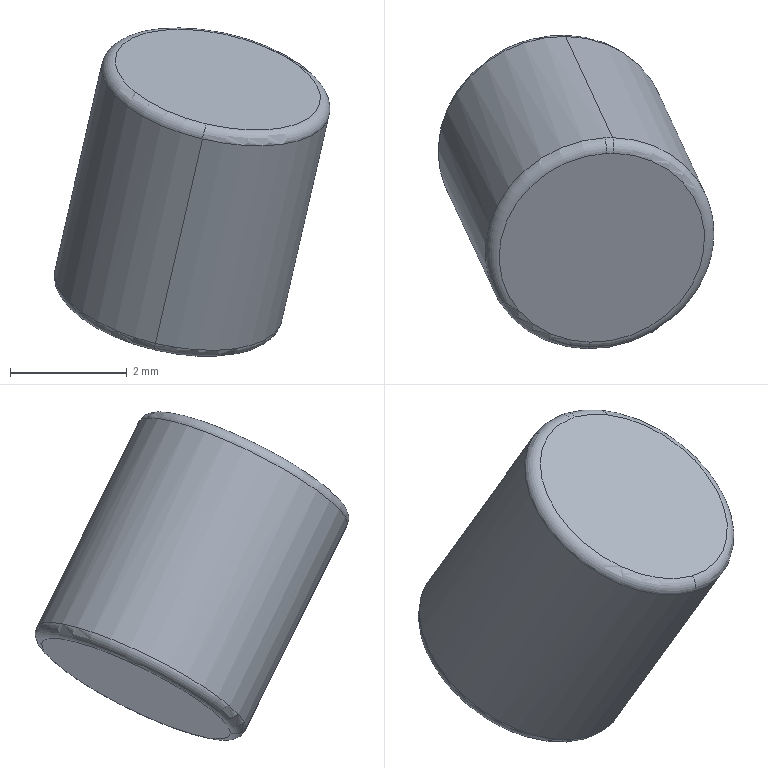Part | SolidWorks | features BaseBody 1 | 1 solid | 9 faces | box 4.732 x 5.384 x 5.638 mm | volume 55.081 mm3 | torus 5 | plane 2 | cylinder 2 | commonest cylinder face diameters 4 x2
STEP:
#1=CARTESIAN_POINT('',(1970.244,-226.347,964.047));
#2=VERTEX_POINT('',#1);
#3=CARTESIAN_POINT('',(1970.524,-223.11,965.592));
#4=VERTEX_POINT('',#3);
#5=CARTESIAN_POINT('',(1970.445,-224.727,964.806));
#6=DIRECTION('',(-0.2015,0.436,-0.8771));
#7=DIRECTION('',(0.9077,0.4197,0.0001618));
#8=AXIS2_PLACEMENT_3D('',#5,#6,#7);
#9=CIRCLE('',#8,1.8);
#10=EDGE_CURVE('',#2,#4,#9,.T.);
#11=ORIENTED_EDGE('',*,*,#10,.T.);
#12=CARTESIAN_POINT('',(1970.492,-222.843,965.504));
#13=VERTEX_POINT('',#12);
#14=CARTESIAN_POINT('',(1970.484,-223.022,965.416));
#15=DIRECTION('',(-0.9785,-0.04965,0.2001));
#16=DIRECTION('',(0.2003,0.,0.9797));
#17=AXIS2_PLACEMENT_3D('',#14,#15,#16);
#18=CIRCLE('',#17,0.2);
#19=EDGE_CURVE('',#4,#13,#18,.T.);
#20=ORIENTED_EDGE('',*,*,#19,.T.);
#21=CARTESIAN_POINT('',(1970.181,-226.439,963.787));
#22=VERTEX_POINT('',#21);
#23=CARTESIAN_POINT('',(1970.405,-224.64,964.63));
#24=DIRECTION('',(-0.2015,0.436,-0.8771));
#25=DIRECTION('',(0.9077,0.4197,0.0001618));
#26=AXIS2_PLACEMENT_3D('',#23,#24,#25);
#27=CIRCLE('',#26,2.);
#28=EDGE_CURVE('',#22,#13,#27,.T.);
#29=ORIENTED_EDGE('',*,*,#28,.F.);
#30=CARTESIAN_POINT('',(1970.203,-226.259,963.872));
#31=DIRECTION('',(0.9731,-0.01332,-0.2301));
#32=DIRECTION('',(0.112,0.8998,0.4216));
#33=AXIS2_PLACEMENT_3D('',#30,#31,#32);
#34=CIRCLE('',#33,0.2);
#35=EDGE_CURVE('',#2,#22,#34,.T.);
#36=ORIENTED_EDGE('',*,*,#35,.F.);
#37=EDGE_LOOP('',(#11,#20,#29,#36));
#38=FACE_OUTER_BOUND('',#37,.T.);
#39=CARTESIAN_POINT('',(1970.405,-224.64,964.63));
#40=DIRECTION('',(-0.2015,0.436,-0.8771));
#41=DIRECTION('',(0.04369,0.8986,0.4367));
#42=AXIS2_PLACEMENT_3D('',#39,#40,#41);
#43=TOROIDAL_SURFACE('',#42,1.8,0.2);
#44=ADVANCED_FACE('',(#38),#43,.T.);
#45=CARTESIAN_POINT('',(1969.357,-224.428,960.188));
#46=VERTEX_POINT('',#45);
#47=CARTESIAN_POINT('',(1969.76,-221.189,961.705));
#48=VERTEX_POINT('',#47);
#49=CARTESIAN_POINT('',(1969.357,-224.428,960.188));
#50=CARTESIAN_POINT('',(1969.158,-224.425,960.235));
#51=CARTESIAN_POINT('',(1968.961,-224.396,960.294));
#52=CARTESIAN_POINT('',(1968.774,-224.341,960.365));
#53=CARTESIAN_POINT('',(1968.404,-224.171,960.534));
#54=CARTESIAN_POINT('',(1968.116,-223.902,960.734));
#55=CARTESIAN_POINT('',(1967.992,-223.735,960.846));
#56=CARTESIAN_POINT('',(1967.802,-223.344,961.084));
#57=CARTESIAN_POINT('',(1967.77,-222.903,961.311));
#58=CARTESIAN_POINT('',(1967.799,-222.666,961.422));
#59=CARTESIAN_POINT('',(1967.939,-222.232,961.605));
#60=CARTESIAN_POINT('',(1968.221,-221.852,961.729));
#61=CARTESIAN_POINT('',(1968.38,-221.692,961.772));
#62=CARTESIAN_POINT('',(1968.731,-221.428,961.823));
#63=CARTESIAN_POINT('',(1969.141,-221.264,961.811));
#64=CARTESIAN_POINT('',(1969.347,-221.211,961.789));
#65=CARTESIAN_POINT('',(1969.555,-221.186,961.754));
#66=CARTESIAN_POINT('',(1969.76,-221.189,961.705));
#67=B_SPLINE_CURVE_WITH_KNOTS('',5,(#49,#50,#51,#52,#53,#54,#55,#56,#57,#58,#59,#60,#61,#62,#63,#64,#65,#66),.UNSPECIFIED.,.F.,.F.,(6,3,3,3,3,6),(0.,0.1813,0.3861,0.6139,0.8137,1.),.UNSPECIFIED.);
#68=EDGE_CURVE('',#46,#48,#67,.T.);
#69=ORIENTED_EDGE('',*,*,#68,.T.);
#70=CARTESIAN_POINT('',(1969.559,-222.808,960.947));
#71=DIRECTION('',(-0.2015,0.436,-0.8771));
#72=DIRECTION('',(0.9077,0.4197,0.0001618));
#73=AXIS2_PLACEMENT_3D('',#70,#71,#72);
#74=CIRCLE('',#73,1.8);
#75=EDGE_CURVE('',#48,#46,#74,.T.);
#76=ORIENTED_EDGE('',*,*,#75,.T.);
#77=EDGE_LOOP('',(#69,#76));
#78=FACE_OUTER_BOUND('',#77,.T.);
#79=CARTESIAN_POINT('',(1969.559,-222.808,960.947));
#80=DIRECTION('',(-0.2015,0.436,-0.8771));
#81=DIRECTION('',(-0.9077,-0.4197,-0.0001618));
#82=AXIS2_PLACEMENT_3D('',#79,#80,#81);
#83=PLANE('',#82);
#84=ADVANCED_FACE('',(#78),#83,.T.);
#85=CARTESIAN_POINT('',(1969.375,-224.695,960.279));
#86=VERTEX_POINT('',#85);
#87=CARTESIAN_POINT('',(1969.397,-224.515,960.363));
#88=DIRECTION('',(-0.9731,0.01332,0.2301));
#89=DIRECTION('',(0.112,0.8998,0.4216));
#90=AXIS2_PLACEMENT_3D('',#87,#88,#89);
#91=CIRCLE('',#90,0.2);
#92=EDGE_CURVE('',#46,#86,#91,.T.);
#93=ORIENTED_EDGE('',*,*,#92,.T.);
#94=CARTESIAN_POINT('',(1969.823,-221.096,961.965));
#95=VERTEX_POINT('',#94);
#96=CARTESIAN_POINT('',(1969.599,-222.896,961.122));
#97=DIRECTION('',(-0.2015,0.436,-0.8771));
#98=DIRECTION('',(0.9077,0.4197,0.0001618));
#99=AXIS2_PLACEMENT_3D('',#96,#97,#98);
#100=CIRCLE('',#99,2.);
#101=EDGE_CURVE('',#86,#95,#100,.T.);
#102=ORIENTED_EDGE('',*,*,#101,.T.);
#103=CARTESIAN_POINT('',(1969.801,-221.276,961.881));
#104=DIRECTION('',(-0.9731,0.01332,0.2301));
#105=DIRECTION('',(0.112,0.8998,0.4216));
#106=AXIS2_PLACEMENT_3D('',#103,#104,#105);
#107=CIRCLE('',#106,0.2);
#108=EDGE_CURVE('',#95,#48,#107,.T.);
#109=ORIENTED_EDGE('',*,*,#108,.T.);
#110=ORIENTED_EDGE('',*,*,#68,.F.);
#111=EDGE_LOOP('',(#93,#102,#109,#110));
#112=FACE_OUTER_BOUND('',#111,.T.);
#113=CARTESIAN_POINT('',(1969.599,-222.896,961.122));
#114=DIRECTION('',(0.2015,-0.436,0.8771));
#115=DIRECTION('',(-0.112,-0.8998,-0.4216));
#116=AXIS2_PLACEMENT_3D('',#113,#114,#115);
#117=TOROIDAL_SURFACE('',#116,1.8,0.2);
#118=ADVANCED_FACE('',(#112),#117,.T.);
#119=ORIENTED_EDGE('',*,*,#108,.F.);
#120=CARTESIAN_POINT('',(1969.599,-222.896,961.122));
#121=DIRECTION('',(-0.2015,0.436,-0.8771));
#122=DIRECTION('',(0.9077,0.4197,0.0001618));
#123=AXIS2_PLACEMENT_3D('',#120,#121,#122);
#124=CIRCLE('',#123,2.);
#125=EDGE_CURVE('',#95,#86,#124,.T.);
#126=ORIENTED_EDGE('',*,*,#125,.T.);
#127=ORIENTED_EDGE('',*,*,#92,.F.);
#128=ORIENTED_EDGE('',*,*,#75,.F.);
#129=EDGE_LOOP('',(#119,#126,#127,#128));
#130=FACE_OUTER_BOUND('',#129,.T.);
#131=CARTESIAN_POINT('',(1969.599,-222.896,961.122));
#132=DIRECTION('',(-0.2015,0.436,-0.8771));
#133=DIRECTION('',(-0.112,-0.8998,-0.4216));
#134=AXIS2_PLACEMENT_3D('',#131,#132,#133);
#135=TOROIDAL_SURFACE('',#134,1.8,0.2);
#136=ADVANCED_FACE('',(#130),#135,.T.);
#137=CARTESIAN_POINT('',(1970.647,-223.107,965.565));
#138=VERTEX_POINT('',#137);
#139=CARTESIAN_POINT('',(1970.445,-224.727,964.806));
#140=DIRECTION('',(-0.2015,0.436,-0.8771));
#141=DIRECTION('',(0.9077,0.4197,0.0001618));
#142=AXIS2_PLACEMENT_3D('',#139,#140,#141);
#143=CIRCLE('',#142,1.8);
#144=EDGE_CURVE('',#138,#2,#143,.T.);
#145=ORIENTED_EDGE('',*,*,#144,.F.);
#146=CARTESIAN_POINT('',(1970.445,-224.727,964.806));
#147=DIRECTION('',(-0.2015,0.436,-0.8771));
#148=DIRECTION('',(0.9077,0.4197,0.0001618));
#149=AXIS2_PLACEMENT_3D('',#146,#147,#148);
#150=CIRCLE('',#149,1.8);
#151=EDGE_CURVE('',#4,#138,#150,.T.);
#152=ORIENTED_EDGE('',*,*,#151,.F.);
#153=ORIENTED_EDGE('',*,*,#10,.F.);
#154=EDGE_LOOP('',(#145,#152,#153));
#155=FACE_OUTER_BOUND('',#154,.T.);
#156=CARTESIAN_POINT('',(1970.445,-224.727,964.806));
#157=DIRECTION('',(-0.2015,0.436,-0.8771));
#158=DIRECTION('',(-0.9077,-0.4197,-0.0001618));
#159=AXIS2_PLACEMENT_3D('',#156,#157,#158);
#160=PLANE('',#159);
#161=ADVANCED_FACE('',(#155),#160,.F.);
#162=CARTESIAN_POINT('',(1969.778,-225.567,962.033));
#163=DIRECTION('',(-0.2015,0.436,-0.8771));
#164=VECTOR('',#163,1000.);
#165=LINE('',#162,#164);
#166=EDGE_CURVE('',#22,#86,#165,.T.);
#167=ORIENTED_EDGE('',*,*,#166,.T.);
#168=ORIENTED_EDGE('',*,*,#125,.F.);
#169=CARTESIAN_POINT('',(1970.629,-222.84,965.474));
#170=VERTEX_POINT('',#169);
#171=CARTESIAN_POINT('',(1970.226,-221.968,963.719));
#172=DIRECTION('',(0.2015,-0.436,0.8771));
#173=VECTOR('',#172,1000.);
#174=LINE('',#171,#173);
#175=EDGE_CURVE('',#95,#170,#174,.T.);
#176=ORIENTED_EDGE('',*,*,#175,.T.);
#177=CARTESIAN_POINT('',(1970.405,-224.64,964.63));
#178=DIRECTION('',(-0.2015,0.436,-0.8771));
#179=DIRECTION('',(0.9077,0.4197,0.0001618));
#180=AXIS2_PLACEMENT_3D('',#177,#178,#179);
#181=CIRCLE('',#180,2.);
#182=EDGE_CURVE('',#170,#22,#181,.T.);
#183=ORIENTED_EDGE('',*,*,#182,.T.);
#184=EDGE_LOOP('',(#167,#168,#176,#183));
#185=FACE_OUTER_BOUND('',#184,.T.);
#186=CARTESIAN_POINT('',(1970.002,-223.768,962.876));
#187=DIRECTION('',(-0.2015,0.436,-0.8771));
#188=DIRECTION('',(-0.112,-0.8998,-0.4216));
#189=AXIS2_PLACEMENT_3D('',#186,#187,#188);
#190=CYLINDRICAL_SURFACE('',#189,2.);
#191=ADVANCED_FACE('',(#185),#190,.T.);
#192=ORIENTED_EDGE('',*,*,#175,.F.);
#193=ORIENTED_EDGE('',*,*,#101,.F.);
#194=ORIENTED_EDGE('',*,*,#166,.F.);
#195=ORIENTED_EDGE('',*,*,#28,.T.);
#196=CARTESIAN_POINT('',(1970.405,-224.64,964.63));
#197=DIRECTION('',(-0.2015,0.436,-0.8771));
#198=DIRECTION('',(0.9077,0.4197,0.0001618));
#199=AXIS2_PLACEMENT_3D('',#196,#197,#198);
#200=CIRCLE('',#199,2.);
#201=EDGE_CURVE('',#13,#170,#200,.T.);
#202=ORIENTED_EDGE('',*,*,#201,.T.);
#203=EDGE_LOOP('',(#192,#193,#194,#195,#202));
#204=FACE_OUTER_BOUND('',#203,.T.);
#205=CARTESIAN_POINT('',(1970.002,-223.768,962.876));
#206=DIRECTION('',(-0.2015,0.436,-0.8771));
#207=DIRECTION('',(-0.112,-0.8998,-0.4216));
#208=AXIS2_PLACEMENT_3D('',#205,#206,#207);
#209=CYLINDRICAL_SURFACE('',#208,2.);
#210=ADVANCED_FACE('',(#204),#209,.T.);
#211=ORIENTED_EDGE('',*,*,#19,.F.);
#212=ORIENTED_EDGE('',*,*,#151,.T.);
#213=CARTESIAN_POINT('',(1970.607,-223.02,965.389));
#214=DIRECTION('',(0.9731,-0.01332,-0.2301));
#215=DIRECTION('',(0.112,0.8998,0.4216));
#216=AXIS2_PLACEMENT_3D('',#213,#214,#215);
#217=CIRCLE('',#216,0.2);
#218=EDGE_CURVE('',#170,#138,#217,.T.);
#219=ORIENTED_EDGE('',*,*,#218,.F.);
#220=ORIENTED_EDGE('',*,*,#201,.F.);
#221=EDGE_LOOP('',(#211,#212,#219,#220));
#222=FACE_OUTER_BOUND('',#221,.T.);
#223=CARTESIAN_POINT('',(1970.405,-224.64,964.63));
#224=DIRECTION('',(-0.2015,0.436,-0.8771));
#225=DIRECTION('',(0.04369,0.8986,0.4367));
#226=AXIS2_PLACEMENT_3D('',#223,#224,#225);
#227=TOROIDAL_SURFACE('',#226,1.8,0.2);
#228=ADVANCED_FACE('',(#222),#227,.T.);
#229=ORIENTED_EDGE('',*,*,#218,.T.);
#230=ORIENTED_EDGE('',*,*,#144,.T.);
#231=ORIENTED_EDGE('',*,*,#35,.T.);
#232=ORIENTED_EDGE('',*,*,#182,.F.);
#233=EDGE_LOOP('',(#229,#230,#231,#232));
#234=FACE_OUTER_BOUND('',#233,.T.);
#235=CARTESIAN_POINT('',(1970.405,-224.64,964.63));
#236=DIRECTION('',(-0.2015,0.436,-0.8771));
#237=DIRECTION('',(-0.112,-0.8998,-0.4216));
#238=AXIS2_PLACEMENT_3D('',#235,#236,#237);
#239=TOROIDAL_SURFACE('',#238,1.8,0.2);
#240=ADVANCED_FACE('',(#234),#239,.T.);
#241=CLOSED_SHELL('',(#44,#84,#118,#136,#161,#191,#210,#228,#240));
#242=MANIFOLD_SOLID_BREP('',#241);
#243=CARTESIAN_POINT('',(0.,0.,0.));
#244=DIRECTION('',(0.,0.,1.));
#245=DIRECTION('',(1.,0.,0.));
#246=AXIS2_PLACEMENT_3D('',#243,#244,#245);
#247=(LENGTH_UNIT()NAMED_UNIT(*)SI_UNIT(.MILLI.,.METRE.));
#248=UNCERTAINTY_MEASURE_WITH_UNIT(LENGTH_MEASURE(0.00001),#247,'','');
#249=(NAMED_UNIT(*)PLANE_ANGLE_UNIT()SI_UNIT($,.RADIAN.));
#250=(NAMED_UNIT(*)SI_UNIT($,.STERADIAN.)SOLID_ANGLE_UNIT());
#251=(GEOMETRIC_REPRESENTATION_CONTEXT(3)GLOBAL_UNCERTAINTY_ASSIGNED_CONTEXT((#248))GLOBAL_UNIT_ASSIGNED_CONTEXT((#247,#249,#250))REPRESENTATION_CONTEXT('',''));
#252=ADVANCED_BREP_SHAPE_REPRESENTATION('',(#242,#246),#251);